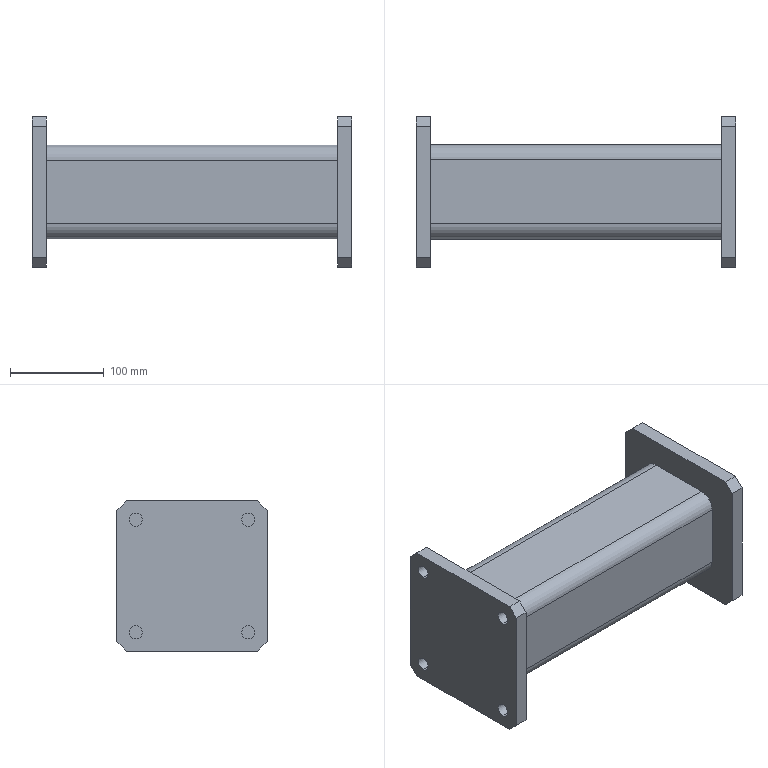Part | SolidWorks | features 3DProfileFeature 1, Extrusion 1, HoleWzd 1, ICE 1, MirrorPattern 1 | 1 solid | 46 faces | box 340 x 160 x 160 mm | volume 1614311 mm3 | plane 30 | cylinder 16 | commonest cylinder face diameters 14 x8 16 x4 32 x4
STEP:
#1=CARTESIAN_POINT('',(0.,140.,-133.));
#2=VERTEX_POINT('',#1);
#3=CARTESIAN_POINT('',(0.,140.,-147.));
#4=VERTEX_POINT('',#3);
#5=CARTESIAN_POINT('',(0.,140.,-140.));
#6=DIRECTION('',(1.,0.,0.));
#7=DIRECTION('',(0.,0.,-1.));
#8=AXIS2_PLACEMENT_3D('',#5,#6,#7);
#9=CIRCLE('',#8,7.);
#10=EDGE_CURVE('',#2,#4,#9,.T.);
#11=ORIENTED_EDGE('',*,*,#10,.F.);
#12=CARTESIAN_POINT('',(15.,140.,-133.));
#13=VERTEX_POINT('',#12);
#14=CARTESIAN_POINT('',(15.,140.,-133.));
#15=DIRECTION('',(1.,0.,0.));
#16=VECTOR('',#15,1000.);
#17=LINE('',#14,#16);
#18=EDGE_CURVE('',#2,#13,#17,.T.);
#19=ORIENTED_EDGE('',*,*,#18,.T.);
#20=CARTESIAN_POINT('',(15.,140.,-147.));
#21=VERTEX_POINT('',#20);
#22=CARTESIAN_POINT('',(15.,140.,-140.));
#23=DIRECTION('',(1.,0.,0.));
#24=DIRECTION('',(0.,0.,-1.));
#25=AXIS2_PLACEMENT_3D('',#22,#23,#24);
#26=CIRCLE('',#25,7.);
#27=EDGE_CURVE('',#13,#21,#26,.T.);
#28=ORIENTED_EDGE('',*,*,#27,.T.);
#29=CARTESIAN_POINT('',(15.,140.,-147.));
#30=DIRECTION('',(1.,0.,0.));
#31=VECTOR('',#30,1000.);
#32=LINE('',#29,#31);
#33=EDGE_CURVE('',#4,#21,#32,.T.);
#34=ORIENTED_EDGE('',*,*,#33,.F.);
#35=EDGE_LOOP('',(#11,#19,#28,#34));
#36=FACE_OUTER_BOUND('',#35,.T.);
#37=CARTESIAN_POINT('',(15.,140.,-140.));
#38=DIRECTION('',(1.,0.,0.));
#39=DIRECTION('',(0.,0.,-1.));
#40=AXIS2_PLACEMENT_3D('',#37,#38,#39);
#41=CYLINDRICAL_SURFACE('',#40,7.);
#42=ADVANCED_FACE('',(#36),#41,.F.);
#43=CARTESIAN_POINT('',(0.,20.,-133.));
#44=VERTEX_POINT('',#43);
#45=CARTESIAN_POINT('',(0.,20.,-147.));
#46=VERTEX_POINT('',#45);
#47=CARTESIAN_POINT('',(0.,20.,-140.));
#48=DIRECTION('',(1.,0.,0.));
#49=DIRECTION('',(0.,0.,-1.));
#50=AXIS2_PLACEMENT_3D('',#47,#48,#49);
#51=CIRCLE('',#50,7.);
#52=EDGE_CURVE('',#44,#46,#51,.T.);
#53=ORIENTED_EDGE('',*,*,#52,.F.);
#54=CARTESIAN_POINT('',(15.,20.,-133.));
#55=VERTEX_POINT('',#54);
#56=CARTESIAN_POINT('',(15.,20.,-133.));
#57=DIRECTION('',(1.,0.,0.));
#58=VECTOR('',#57,1000.);
#59=LINE('',#56,#58);
#60=EDGE_CURVE('',#44,#55,#59,.T.);
#61=ORIENTED_EDGE('',*,*,#60,.T.);
#62=CARTESIAN_POINT('',(15.,20.,-147.));
#63=VERTEX_POINT('',#62);
#64=CARTESIAN_POINT('',(15.,20.,-140.));
#65=DIRECTION('',(1.,0.,0.));
#66=DIRECTION('',(0.,0.,-1.));
#67=AXIS2_PLACEMENT_3D('',#64,#65,#66);
#68=CIRCLE('',#67,7.);
#69=EDGE_CURVE('',#55,#63,#68,.T.);
#70=ORIENTED_EDGE('',*,*,#69,.T.);
#71=CARTESIAN_POINT('',(15.,20.,-147.));
#72=DIRECTION('',(1.,0.,0.));
#73=VECTOR('',#72,1000.);
#74=LINE('',#71,#73);
#75=EDGE_CURVE('',#46,#63,#74,.T.);
#76=ORIENTED_EDGE('',*,*,#75,.F.);
#77=EDGE_LOOP('',(#53,#61,#70,#76));
#78=FACE_OUTER_BOUND('',#77,.T.);
#79=CARTESIAN_POINT('',(15.,20.,-140.));
#80=DIRECTION('',(1.,0.,0.));
#81=DIRECTION('',(0.,0.,-1.));
#82=AXIS2_PLACEMENT_3D('',#79,#80,#81);
#83=CYLINDRICAL_SURFACE('',#82,7.);
#84=ADVANCED_FACE('',(#78),#83,.F.);
#85=CARTESIAN_POINT('',(0.,140.,-13.));
#86=VERTEX_POINT('',#85);
#87=CARTESIAN_POINT('',(0.,140.,-27.));
#88=VERTEX_POINT('',#87);
#89=CARTESIAN_POINT('',(0.,140.,-20.));
#90=DIRECTION('',(1.,0.,0.));
#91=DIRECTION('',(0.,0.,-1.));
#92=AXIS2_PLACEMENT_3D('',#89,#90,#91);
#93=CIRCLE('',#92,7.);
#94=EDGE_CURVE('',#86,#88,#93,.T.);
#95=ORIENTED_EDGE('',*,*,#94,.F.);
#96=CARTESIAN_POINT('',(15.,140.,-13.));
#97=VERTEX_POINT('',#96);
#98=CARTESIAN_POINT('',(15.,140.,-13.));
#99=DIRECTION('',(1.,0.,0.));
#100=VECTOR('',#99,1000.);
#101=LINE('',#98,#100);
#102=EDGE_CURVE('',#86,#97,#101,.T.);
#103=ORIENTED_EDGE('',*,*,#102,.T.);
#104=CARTESIAN_POINT('',(15.,140.,-27.));
#105=VERTEX_POINT('',#104);
#106=CARTESIAN_POINT('',(15.,140.,-20.));
#107=DIRECTION('',(1.,0.,0.));
#108=DIRECTION('',(0.,0.,-1.));
#109=AXIS2_PLACEMENT_3D('',#106,#107,#108);
#110=CIRCLE('',#109,7.);
#111=EDGE_CURVE('',#97,#105,#110,.T.);
#112=ORIENTED_EDGE('',*,*,#111,.T.);
#113=CARTESIAN_POINT('',(15.,140.,-27.));
#114=DIRECTION('',(1.,0.,0.));
#115=VECTOR('',#114,1000.);
#116=LINE('',#113,#115);
#117=EDGE_CURVE('',#88,#105,#116,.T.);
#118=ORIENTED_EDGE('',*,*,#117,.F.);
#119=EDGE_LOOP('',(#95,#103,#112,#118));
#120=FACE_OUTER_BOUND('',#119,.T.);
#121=CARTESIAN_POINT('',(15.,140.,-20.));
#122=DIRECTION('',(1.,0.,0.));
#123=DIRECTION('',(0.,0.,-1.));
#124=AXIS2_PLACEMENT_3D('',#121,#122,#123);
#125=CYLINDRICAL_SURFACE('',#124,7.);
#126=ADVANCED_FACE('',(#120),#125,.F.);
#127=CARTESIAN_POINT('',(0.,20.,-13.));
#128=VERTEX_POINT('',#127);
#129=CARTESIAN_POINT('',(0.,20.,-27.));
#130=VERTEX_POINT('',#129);
#131=CARTESIAN_POINT('',(0.,20.,-20.));
#132=DIRECTION('',(1.,0.,0.));
#133=DIRECTION('',(0.,0.,-1.));
#134=AXIS2_PLACEMENT_3D('',#131,#132,#133);
#135=CIRCLE('',#134,7.);
#136=EDGE_CURVE('',#128,#130,#135,.T.);
#137=ORIENTED_EDGE('',*,*,#136,.F.);
#138=CARTESIAN_POINT('',(15.,20.,-13.));
#139=VERTEX_POINT('',#138);
#140=CARTESIAN_POINT('',(15.,20.,-13.));
#141=DIRECTION('',(1.,0.,0.));
#142=VECTOR('',#141,1000.);
#143=LINE('',#140,#142);
#144=EDGE_CURVE('',#128,#139,#143,.T.);
#145=ORIENTED_EDGE('',*,*,#144,.T.);
#146=CARTESIAN_POINT('',(15.,20.,-27.));
#147=VERTEX_POINT('',#146);
#148=CARTESIAN_POINT('',(15.,20.,-20.));
#149=DIRECTION('',(1.,0.,0.));
#150=DIRECTION('',(0.,0.,-1.));
#151=AXIS2_PLACEMENT_3D('',#148,#149,#150);
#152=CIRCLE('',#151,7.);
#153=EDGE_CURVE('',#139,#147,#152,.T.);
#154=ORIENTED_EDGE('',*,*,#153,.T.);
#155=CARTESIAN_POINT('',(15.,20.,-27.));
#156=DIRECTION('',(1.,0.,0.));
#157=VECTOR('',#156,1000.);
#158=LINE('',#155,#157);
#159=EDGE_CURVE('',#130,#147,#158,.T.);
#160=ORIENTED_EDGE('',*,*,#159,.F.);
#161=EDGE_LOOP('',(#137,#145,#154,#160));
#162=FACE_OUTER_BOUND('',#161,.T.);
#163=CARTESIAN_POINT('',(15.,20.,-20.));
#164=DIRECTION('',(1.,0.,0.));
#165=DIRECTION('',(0.,0.,-1.));
#166=AXIS2_PLACEMENT_3D('',#163,#164,#165);
#167=CYLINDRICAL_SURFACE('',#166,7.);
#168=ADVANCED_FACE('',(#162),#167,.F.);
#169=CARTESIAN_POINT('',(15.,140.,-140.));
#170=DIRECTION('',(1.,0.,0.));
#171=DIRECTION('',(0.,0.,-1.));
#172=AXIS2_PLACEMENT_3D('',#169,#170,#171);
#173=CIRCLE('',#172,7.);
#174=EDGE_CURVE('',#21,#13,#173,.T.);
#175=ORIENTED_EDGE('',*,*,#174,.F.);
#176=ORIENTED_EDGE('',*,*,#27,.F.);
#177=EDGE_LOOP('',(#175,#176));
#178=FACE_BOUND('',#177,.T.);
#179=CARTESIAN_POINT('',(15.,20.,-140.));
#180=DIRECTION('',(1.,0.,0.));
#181=DIRECTION('',(0.,0.,-1.));
#182=AXIS2_PLACEMENT_3D('',#179,#180,#181);
#183=CIRCLE('',#182,7.);
#184=EDGE_CURVE('',#63,#55,#183,.T.);
#185=ORIENTED_EDGE('',*,*,#184,.F.);
#186=ORIENTED_EDGE('',*,*,#69,.F.);
#187=EDGE_LOOP('',(#185,#186));
#188=FACE_BOUND('',#187,.T.);
#189=CARTESIAN_POINT('',(15.,140.,-20.));
#190=DIRECTION('',(1.,0.,0.));
#191=DIRECTION('',(0.,0.,-1.));
#192=AXIS2_PLACEMENT_3D('',#189,#190,#191);
#193=CIRCLE('',#192,7.);
#194=EDGE_CURVE('',#105,#97,#193,.T.);
#195=ORIENTED_EDGE('',*,*,#194,.F.);
#196=ORIENTED_EDGE('',*,*,#111,.F.);
#197=EDGE_LOOP('',(#195,#196));
#198=FACE_BOUND('',#197,.T.);
#199=CARTESIAN_POINT('',(15.,20.,-20.));
#200=DIRECTION('',(1.,0.,0.));
#201=DIRECTION('',(0.,0.,-1.));
#202=AXIS2_PLACEMENT_3D('',#199,#200,#201);
#203=CIRCLE('',#202,7.);
#204=EDGE_CURVE('',#147,#139,#203,.T.);
#205=ORIENTED_EDGE('',*,*,#204,.F.);
#206=ORIENTED_EDGE('',*,*,#153,.F.);
#207=EDGE_LOOP('',(#205,#206));
#208=FACE_BOUND('',#207,.T.);
#209=CARTESIAN_POINT('',(15.,160.,-150.));
#210=VERTEX_POINT('',#209);
#211=CARTESIAN_POINT('',(15.,160.,-10.));
#212=VERTEX_POINT('',#211);
#213=CARTESIAN_POINT('',(15.,160.,-10.));
#214=DIRECTION('',(0.,0.,1.));
#215=VECTOR('',#214,1000.);
#216=LINE('',#213,#215);
#217=EDGE_CURVE('',#210,#212,#216,.T.);
#218=ORIENTED_EDGE('',*,*,#217,.T.);
#219=CARTESIAN_POINT('',(15.,150.,0.));
#220=VERTEX_POINT('',#219);
#221=CARTESIAN_POINT('',(15.,150.,0.));
#222=DIRECTION('',(0.,-0.7071,0.7071));
#223=VECTOR('',#222,1000.);
#224=LINE('',#221,#223);
#225=EDGE_CURVE('',#212,#220,#224,.T.);
#226=ORIENTED_EDGE('',*,*,#225,.T.);
#227=CARTESIAN_POINT('',(15.,10.,0.));
#228=VERTEX_POINT('',#227);
#229=CARTESIAN_POINT('',(15.,10.,0.));
#230=DIRECTION('',(0.,-1.,0.));
#231=VECTOR('',#230,1000.);
#232=LINE('',#229,#231);
#233=EDGE_CURVE('',#220,#228,#232,.T.);
#234=ORIENTED_EDGE('',*,*,#233,.T.);
#235=CARTESIAN_POINT('',(15.,0.,-10.));
#236=VERTEX_POINT('',#235);
#237=CARTESIAN_POINT('',(15.,0.,-10.));
#238=DIRECTION('',(0.,-0.7071,-0.7071));
#239=VECTOR('',#238,1000.);
#240=LINE('',#237,#239);
#241=EDGE_CURVE('',#228,#236,#240,.T.);
#242=ORIENTED_EDGE('',*,*,#241,.T.);
#243=CARTESIAN_POINT('',(15.,0.,-150.));
#244=VERTEX_POINT('',#243);
#245=CARTESIAN_POINT('',(15.,0.,-10.));
#246=DIRECTION('',(0.,0.,-1.));
#247=VECTOR('',#246,1000.);
#248=LINE('',#245,#247);
#249=EDGE_CURVE('',#236,#244,#248,.T.);
#250=ORIENTED_EDGE('',*,*,#249,.T.);
#251=CARTESIAN_POINT('',(15.,10.,-160.));
#252=VERTEX_POINT('',#251);
#253=CARTESIAN_POINT('',(15.,0.,-150.));
#254=DIRECTION('',(0.,0.7071,-0.7071));
#255=VECTOR('',#254,1000.);
#256=LINE('',#253,#255);
#257=EDGE_CURVE('',#244,#252,#256,.T.);
#258=ORIENTED_EDGE('',*,*,#257,.T.);
#259=CARTESIAN_POINT('',(15.,150.,-160.));
#260=VERTEX_POINT('',#259);
#261=CARTESIAN_POINT('',(15.,10.,-160.));
#262=DIRECTION('',(0.,1.,0.));
#263=VECTOR('',#262,1000.);
#264=LINE('',#261,#263);
#265=EDGE_CURVE('',#252,#260,#264,.T.);
#266=ORIENTED_EDGE('',*,*,#265,.T.);
#267=CARTESIAN_POINT('',(15.,150.,-160.));
#268=DIRECTION('',(0.,0.7071,0.7071));
#269=VECTOR('',#268,1000.);
#270=LINE('',#267,#269);
#271=EDGE_CURVE('',#260,#210,#270,.T.);
#272=ORIENTED_EDGE('',*,*,#271,.T.);
#273=EDGE_LOOP('',(#218,#226,#234,#242,#250,#258,#266,#272));
#274=FACE_OUTER_BOUND('',#273,.T.);
#275=CARTESIAN_POINT('',(15.,130.,-114.));
#276=VERTEX_POINT('',#275);
#277=CARTESIAN_POINT('',(15.,130.,-46.));
#278=VERTEX_POINT('',#277);
#279=CARTESIAN_POINT('',(15.,130.,-46.));
#280=DIRECTION('',(0.,0.,1.));
#281=VECTOR('',#280,1000.);
#282=LINE('',#279,#281);
#283=EDGE_CURVE('',#276,#278,#282,.T.);
#284=ORIENTED_EDGE('',*,*,#283,.F.);
#285=CARTESIAN_POINT('',(15.,114.,-130.));
#286=VERTEX_POINT('',#285);
#287=CARTESIAN_POINT('',(15.,114.,-114.));
#288=DIRECTION('',(1.,0.,0.));
#289=DIRECTION('',(0.,0.,1.));
#290=AXIS2_PLACEMENT_3D('',#287,#288,#289);
#291=CIRCLE('',#290,16.);
#292=EDGE_CURVE('',#286,#276,#291,.T.);
#293=ORIENTED_EDGE('',*,*,#292,.F.);
#294=CARTESIAN_POINT('',(15.,46.,-130.));
#295=VERTEX_POINT('',#294);
#296=CARTESIAN_POINT('',(15.,114.,-130.));
#297=DIRECTION('',(0.,1.,0.));
#298=VECTOR('',#297,1000.);
#299=LINE('',#296,#298);
#300=EDGE_CURVE('',#295,#286,#299,.T.);
#301=ORIENTED_EDGE('',*,*,#300,.F.);
#302=CARTESIAN_POINT('',(15.,30.,-114.));
#303=VERTEX_POINT('',#302);
#304=CARTESIAN_POINT('',(15.,46.,-114.));
#305=DIRECTION('',(1.,0.,0.));
#306=DIRECTION('',(0.,0.,1.));
#307=AXIS2_PLACEMENT_3D('',#304,#305,#306);
#308=CIRCLE('',#307,16.);
#309=EDGE_CURVE('',#303,#295,#308,.T.);
#310=ORIENTED_EDGE('',*,*,#309,.F.);
#311=CARTESIAN_POINT('',(15.,30.,-46.));
#312=VERTEX_POINT('',#311);
#313=CARTESIAN_POINT('',(15.,30.,-46.));
#314=DIRECTION('',(0.,0.,-1.));
#315=VECTOR('',#314,1000.);
#316=LINE('',#313,#315);
#317=EDGE_CURVE('',#312,#303,#316,.T.);
#318=ORIENTED_EDGE('',*,*,#317,.F.);
#319=CARTESIAN_POINT('',(15.,46.,-30.));
#320=VERTEX_POINT('',#319);
#321=CARTESIAN_POINT('',(15.,46.,-46.));
#322=DIRECTION('',(1.,0.,0.));
#323=DIRECTION('',(0.,0.,1.));
#324=AXIS2_PLACEMENT_3D('',#321,#322,#323);
#325=CIRCLE('',#324,16.);
#326=EDGE_CURVE('',#320,#312,#325,.T.);
#327=ORIENTED_EDGE('',*,*,#326,.F.);
#328=CARTESIAN_POINT('',(15.,114.,-30.));
#329=VERTEX_POINT('',#328);
#330=CARTESIAN_POINT('',(15.,114.,-30.));
#331=DIRECTION('',(0.,-1.,0.));
#332=VECTOR('',#331,1000.);
#333=LINE('',#330,#332);
#334=EDGE_CURVE('',#329,#320,#333,.T.);
#335=ORIENTED_EDGE('',*,*,#334,.F.);
#336=CARTESIAN_POINT('',(15.,114.,-46.));
#337=DIRECTION('',(1.,0.,0.));
#338=DIRECTION('',(0.,0.,1.));
#339=AXIS2_PLACEMENT_3D('',#336,#337,#338);
#340=CIRCLE('',#339,16.);
#341=EDGE_CURVE('',#278,#329,#340,.T.);
#342=ORIENTED_EDGE('',*,*,#341,.F.);
#343=EDGE_LOOP('',(#284,#293,#301,#310,#318,#327,#335,#342));
#344=FACE_BOUND('',#343,.T.);
#345=CARTESIAN_POINT('',(15.,160.,-160.));
#346=DIRECTION('',(1.,0.,0.));
#347=DIRECTION('',(0.,0.,-1.));
#348=AXIS2_PLACEMENT_3D('',#345,#346,#347);
#349=PLANE('',#348);
#350=ADVANCED_FACE('',(#178,#188,#198,#208,#274,#344),#349,.T.);
#351=CARTESIAN_POINT('',(0.,160.,-150.));
#352=VERTEX_POINT('',#351);
#353=CARTESIAN_POINT('',(0.,160.,-10.));
#354=VERTEX_POINT('',#353);
#355=CARTESIAN_POINT('',(0.,160.,-10.));
#356=DIRECTION('',(0.,0.,1.));
#357=VECTOR('',#356,1000.);
#358=LINE('',#355,#357);
#359=EDGE_CURVE('',#352,#354,#358,.T.);
#360=ORIENTED_EDGE('',*,*,#359,.T.);
#361=CARTESIAN_POINT('',(15.,160.,-10.));
#362=DIRECTION('',(-1.,0.,0.));
#363=VECTOR('',#362,1000.);
#364=LINE('',#361,#363);
#365=EDGE_CURVE('',#212,#354,#364,.T.);
#366=ORIENTED_EDGE('',*,*,#365,.F.);
#367=ORIENTED_EDGE('',*,*,#217,.F.);
#368=CARTESIAN_POINT('',(15.,160.,-150.));
#369=DIRECTION('',(-1.,0.,0.));
#370=VECTOR('',#369,1000.);
#371=LINE('',#368,#370);
#372=EDGE_CURVE('',#210,#352,#371,.T.);
#373=ORIENTED_EDGE('',*,*,#372,.T.);
#374=EDGE_LOOP('',(#360,#366,#367,#373));
#375=FACE_OUTER_BOUND('',#374,.T.);
#376=CARTESIAN_POINT('',(15.,160.,-10.));
#377=DIRECTION('',(0.,-1.,0.));
#378=DIRECTION('',(0.,0.,-1.));
#379=AXIS2_PLACEMENT_3D('',#376,#377,#378);
#380=PLANE('',#379);
#381=ADVANCED_FACE('',(#375),#380,.F.);
#382=CARTESIAN_POINT('',(0.,150.,0.));
#383=VERTEX_POINT('',#382);
#384=CARTESIAN_POINT('',(0.,150.,0.));
#385=DIRECTION('',(0.,-0.7071,0.7071));
#386=VECTOR('',#385,1000.);
#387=LINE('',#384,#386);
#388=EDGE_CURVE('',#354,#383,#387,.T.);
#389=ORIENTED_EDGE('',*,*,#388,.T.);
#390=CARTESIAN_POINT('',(15.,150.,0.));
#391=DIRECTION('',(-1.,0.,0.));
#392=VECTOR('',#391,1000.);
#393=LINE('',#390,#392);
#394=EDGE_CURVE('',#220,#383,#393,.T.);
#395=ORIENTED_EDGE('',*,*,#394,.F.);
#396=ORIENTED_EDGE('',*,*,#225,.F.);
#397=ORIENTED_EDGE('',*,*,#365,.T.);
#398=EDGE_LOOP('',(#389,#395,#396,#397));
#399=FACE_OUTER_BOUND('',#398,.T.);
#400=CARTESIAN_POINT('',(15.,150.,0.));
#401=DIRECTION('',(0.,-0.7071,-0.7071));
#402=DIRECTION('',(0.,0.7071,-0.7071));
#403=AXIS2_PLACEMENT_3D('',#400,#401,#402);
#404=PLANE('',#403);
#405=ADVANCED_FACE('',(#399),#404,.F.);
#406=CARTESIAN_POINT('',(0.,10.,0.));
#407=VERTEX_POINT('',#406);
#408=CARTESIAN_POINT('',(0.,10.,0.));
#409=DIRECTION('',(0.,-1.,0.));
#410=VECTOR('',#409,1000.);
#411=LINE('',#408,#410);
#412=EDGE_CURVE('',#383,#407,#411,.T.);
#413=ORIENTED_EDGE('',*,*,#412,.T.);
#414=CARTESIAN_POINT('',(15.,10.,0.));
#415=DIRECTION('',(-1.,0.,0.));
#416=VECTOR('',#415,1000.);
#417=LINE('',#414,#416);
#418=EDGE_CURVE('',#228,#407,#417,.T.);
#419=ORIENTED_EDGE('',*,*,#418,.F.);
#420=ORIENTED_EDGE('',*,*,#233,.F.);
#421=ORIENTED_EDGE('',*,*,#394,.T.);
#422=EDGE_LOOP('',(#413,#419,#420,#421));
#423=FACE_OUTER_BOUND('',#422,.T.);
#424=CARTESIAN_POINT('',(15.,10.,0.));
#425=DIRECTION('',(0.,0.,-1.));
#426=DIRECTION('',(-1.,0.,0.));
#427=AXIS2_PLACEMENT_3D('',#424,#425,#426);
#428=PLANE('',#427);
#429=ADVANCED_FACE('',(#423),#428,.F.);
#430=CARTESIAN_POINT('',(0.,0.,-10.));
#431=VERTEX_POINT('',#430);
#432=CARTESIAN_POINT('',(0.,0.,-10.));
#433=DIRECTION('',(0.,-0.7071,-0.7071));
#434=VECTOR('',#433,1000.);
#435=LINE('',#432,#434);
#436=EDGE_CURVE('',#407,#431,#435,.T.);
#437=ORIENTED_EDGE('',*,*,#436,.T.);
#438=CARTESIAN_POINT('',(15.,0.,-10.));
#439=DIRECTION('',(-1.,0.,0.));
#440=VECTOR('',#439,1000.);
#441=LINE('',#438,#440);
#442=EDGE_CURVE('',#236,#431,#441,.T.);
#443=ORIENTED_EDGE('',*,*,#442,.F.);
#444=ORIENTED_EDGE('',*,*,#241,.F.);
#445=ORIENTED_EDGE('',*,*,#418,.T.);
#446=EDGE_LOOP('',(#437,#443,#444,#445));
#447=FACE_OUTER_BOUND('',#446,.T.);
#448=CARTESIAN_POINT('',(15.,0.,-10.));
#449=DIRECTION('',(0.,0.7071,-0.7071));
#450=DIRECTION('',(0.,0.7071,0.7071));
#451=AXIS2_PLACEMENT_3D('',#448,#449,#450);
#452=PLANE('',#451);
#453=ADVANCED_FACE('',(#447),#452,.F.);
#454=CARTESIAN_POINT('',(0.,0.,-150.));
#455=VERTEX_POINT('',#454);
#456=CARTESIAN_POINT('',(0.,0.,-10.));
#457=DIRECTION('',(0.,0.,-1.));
#458=VECTOR('',#457,1000.);
#459=LINE('',#456,#458);
#460=EDGE_CURVE('',#431,#455,#459,.T.);
#461=ORIENTED_EDGE('',*,*,#460,.T.);
#462=CARTESIAN_POINT('',(15.,0.,-150.));
#463=DIRECTION('',(-1.,0.,0.));
#464=VECTOR('',#463,1000.);
#465=LINE('',#462,#464);
#466=EDGE_CURVE('',#244,#455,#465,.T.);
#467=ORIENTED_EDGE('',*,*,#466,.F.);
#468=ORIENTED_EDGE('',*,*,#249,.F.);
#469=ORIENTED_EDGE('',*,*,#442,.T.);
#470=EDGE_LOOP('',(#461,#467,#468,#469));
#471=FACE_OUTER_BOUND('',#470,.T.);
#472=CARTESIAN_POINT('',(15.,0.,-10.));
#473=DIRECTION('',(0.,1.,0.));
#474=DIRECTION('',(0.,0.,1.));
#475=AXIS2_PLACEMENT_3D('',#472,#473,#474);
#476=PLANE('',#475);
#477=ADVANCED_FACE('',(#471),#476,.F.);
#478=CARTESIAN_POINT('',(0.,10.,-160.));
#479=VERTEX_POINT('',#478);
#480=CARTESIAN_POINT('',(0.,0.,-150.));
#481=DIRECTION('',(0.,0.7071,-0.7071));
#482=VECTOR('',#481,1000.);
#483=LINE('',#480,#482);
#484=EDGE_CURVE('',#455,#479,#483,.T.);
#485=ORIENTED_EDGE('',*,*,#484,.T.);
#486=CARTESIAN_POINT('',(15.,10.,-160.));
#487=DIRECTION('',(-1.,0.,0.));
#488=VECTOR('',#487,1000.);
#489=LINE('',#486,#488);
#490=EDGE_CURVE('',#252,#479,#489,.T.);
#491=ORIENTED_EDGE('',*,*,#490,.F.);
#492=ORIENTED_EDGE('',*,*,#257,.F.);
#493=ORIENTED_EDGE('',*,*,#466,.T.);
#494=EDGE_LOOP('',(#485,#491,#492,#493));
#495=FACE_OUTER_BOUND('',#494,.T.);
#496=CARTESIAN_POINT('',(15.,0.,-150.));
#497=DIRECTION('',(0.,0.7071,0.7071));
#498=DIRECTION('',(0.,-0.7071,0.7071));
#499=AXIS2_PLACEMENT_3D('',#496,#497,#498);
#500=PLANE('',#499);
#501=ADVANCED_FACE('',(#495),#500,.F.);
#502=CARTESIAN_POINT('',(0.,150.,-160.));
#503=VERTEX_POINT('',#502);
#504=CARTESIAN_POINT('',(0.,10.,-160.));
#505=DIRECTION('',(0.,1.,0.));
#506=VECTOR('',#505,1000.);
#507=LINE('',#504,#506);
#508=EDGE_CURVE('',#479,#503,#507,.T.);
#509=ORIENTED_EDGE('',*,*,#508,.T.);
#510=CARTESIAN_POINT('',(15.,150.,-160.));
#511=DIRECTION('',(-1.,0.,0.));
#512=VECTOR('',#511,1000.);
#513=LINE('',#510,#512);
#514=EDGE_CURVE('',#260,#503,#513,.T.);
#515=ORIENTED_EDGE('',*,*,#514,.F.);
#516=ORIENTED_EDGE('',*,*,#265,.F.);
#517=ORIENTED_EDGE('',*,*,#490,.T.);
#518=EDGE_LOOP('',(#509,#515,#516,#517));
#519=FACE_OUTER_BOUND('',#518,.T.);
#520=CARTESIAN_POINT('',(15.,10.,-160.));
#521=DIRECTION('',(0.,0.,1.));
#522=DIRECTION('',(1.,0.,0.));
#523=AXIS2_PLACEMENT_3D('',#520,#521,#522);
#524=PLANE('',#523);
#525=ADVANCED_FACE('',(#519),#524,.F.);
#526=CARTESIAN_POINT('',(0.,150.,-160.));
#527=DIRECTION('',(0.,0.7071,0.7071));
#528=VECTOR('',#527,1000.);
#529=LINE('',#526,#528);
#530=EDGE_CURVE('',#503,#352,#529,.T.);
#531=ORIENTED_EDGE('',*,*,#530,.T.);
#532=ORIENTED_EDGE('',*,*,#372,.F.);
#533=ORIENTED_EDGE('',*,*,#271,.F.);
#534=ORIENTED_EDGE('',*,*,#514,.T.);
#535=EDGE_LOOP('',(#531,#532,#533,#534));
#536=FACE_OUTER_BOUND('',#535,.T.);
#537=CARTESIAN_POINT('',(15.,150.,-160.));
#538=DIRECTION('',(0.,-0.7071,0.7071));
#539=DIRECTION('',(0.,-0.7071,-0.7071));
#540=AXIS2_PLACEMENT_3D('',#537,#538,#539);
#541=PLANE('',#540);
#542=ADVANCED_FACE('',(#536),#541,.F.);
#543=CARTESIAN_POINT('',(0.,140.,-140.));
#544=DIRECTION('',(1.,0.,0.));
#545=DIRECTION('',(0.,0.,-1.));
#546=AXIS2_PLACEMENT_3D('',#543,#544,#545);
#547=CIRCLE('',#546,7.);
#548=EDGE_CURVE('',#4,#2,#547,.T.);
#549=ORIENTED_EDGE('',*,*,#548,.T.);
#550=ORIENTED_EDGE('',*,*,#10,.T.);
#551=EDGE_LOOP('',(#549,#550));
#552=FACE_BOUND('',#551,.T.);
#553=CARTESIAN_POINT('',(0.,20.,-140.));
#554=DIRECTION('',(1.,0.,0.));
#555=DIRECTION('',(0.,0.,-1.));
#556=AXIS2_PLACEMENT_3D('',#553,#554,#555);
#557=CIRCLE('',#556,7.);
#558=EDGE_CURVE('',#46,#44,#557,.T.);
#559=ORIENTED_EDGE('',*,*,#558,.T.);
#560=ORIENTED_EDGE('',*,*,#52,.T.);
#561=EDGE_LOOP('',(#559,#560));
#562=FACE_BOUND('',#561,.T.);
#563=CARTESIAN_POINT('',(0.,140.,-20.));
#564=DIRECTION('',(1.,0.,0.));
#565=DIRECTION('',(0.,0.,-1.));
#566=AXIS2_PLACEMENT_3D('',#563,#564,#565);
#567=CIRCLE('',#566,7.);
#568=EDGE_CURVE('',#88,#86,#567,.T.);
#569=ORIENTED_EDGE('',*,*,#568,.T.);
#570=ORIENTED_EDGE('',*,*,#94,.T.);
#571=EDGE_LOOP('',(#569,#570));
#572=FACE_BOUND('',#571,.T.);
#573=CARTESIAN_POINT('',(0.,20.,-20.));
#574=DIRECTION('',(1.,0.,0.));
#575=DIRECTION('',(0.,0.,-1.));
#576=AXIS2_PLACEMENT_3D('',#573,#574,#575);
#577=CIRCLE('',#576,7.);
#578=EDGE_CURVE('',#130,#128,#577,.T.);
#579=ORIENTED_EDGE('',*,*,#578,.T.);
#580=ORIENTED_EDGE('',*,*,#136,.T.);
#581=EDGE_LOOP('',(#579,#580));
#582=FACE_BOUND('',#581,.T.);
#583=ORIENTED_EDGE('',*,*,#359,.F.);
#584=ORIENTED_EDGE('',*,*,#530,.F.);
#585=ORIENTED_EDGE('',*,*,#508,.F.);
#586=ORIENTED_EDGE('',*,*,#484,.F.);
#587=ORIENTED_EDGE('',*,*,#460,.F.);
#588=ORIENTED_EDGE('',*,*,#436,.F.);
#589=ORIENTED_EDGE('',*,*,#412,.F.);
#590=ORIENTED_EDGE('',*,*,#388,.F.);
#591=EDGE_LOOP('',(#583,#584,#585,#586,#587,#588,#589,#590));
#592=FACE_OUTER_BOUND('',#591,.T.);
#593=CARTESIAN_POINT('',(0.,160.,-160.));
#594=DIRECTION('',(1.,0.,0.));
#595=DIRECTION('',(0.,0.,-1.));
#596=AXIS2_PLACEMENT_3D('',#593,#594,#595);
#597=PLANE('',#596);
#598=ADVANCED_FACE('',(#552,#562,#572,#582,#592),#597,.F.);
#599=ORIENTED_EDGE('',*,*,#292,.T.);
#600=CARTESIAN_POINT('',(325.,130.,-114.));
#601=VERTEX_POINT('',#600);
#602=CARTESIAN_POINT('',(325.,130.,-114.));
#603=DIRECTION('',(-1.,0.,0.));
#604=VECTOR('',#603,1000.);
#605=LINE('',#602,#604);
#606=EDGE_CURVE('',#601,#276,#605,.T.);
#607=ORIENTED_EDGE('',*,*,#606,.F.);
#608=CARTESIAN_POINT('',(325.,114.,-130.));
#609=VERTEX_POINT('',#608);
#610=CARTESIAN_POINT('',(325.,114.,-114.));
#611=DIRECTION('',(1.,0.,0.));
#612=DIRECTION('',(0.,0.,1.));
#613=AXIS2_PLACEMENT_3D('',#610,#611,#612);
#614=CIRCLE('',#613,16.);
#615=EDGE_CURVE('',#609,#601,#614,.T.);
#616=ORIENTED_EDGE('',*,*,#615,.F.);
#617=CARTESIAN_POINT('',(325.,114.,-130.));
#618=DIRECTION('',(-1.,0.,0.));
#619=VECTOR('',#618,1000.);
#620=LINE('',#617,#619);
#621=EDGE_CURVE('',#609,#286,#620,.T.);
#622=ORIENTED_EDGE('',*,*,#621,.T.);
#623=EDGE_LOOP('',(#599,#607,#616,#622));
#624=FACE_OUTER_BOUND('',#623,.T.);
#625=CARTESIAN_POINT('',(325.,114.,-114.));
#626=DIRECTION('',(-1.,0.,0.));
#627=DIRECTION('',(0.,0.,1.));
#628=AXIS2_PLACEMENT_3D('',#625,#626,#627);
#629=CYLINDRICAL_SURFACE('',#628,16.);
#630=ADVANCED_FACE('',(#624),#629,.T.);
#631=ORIENTED_EDGE('',*,*,#283,.T.);
#632=CARTESIAN_POINT('',(325.,130.,-46.));
#633=VERTEX_POINT('',#632);
#634=CARTESIAN_POINT('',(325.,130.,-46.));
#635=DIRECTION('',(-1.,0.,0.));
#636=VECTOR('',#635,1000.);
#637=LINE('',#634,#636);
#638=EDGE_CURVE('',#633,#278,#637,.T.);
#639=ORIENTED_EDGE('',*,*,#638,.F.);
#640=CARTESIAN_POINT('',(325.,130.,-46.));
#641=DIRECTION('',(0.,0.,1.));
#642=VECTOR('',#641,1000.);
#643=LINE('',#640,#642);
#644=EDGE_CURVE('',#601,#633,#643,.T.);
#645=ORIENTED_EDGE('',*,*,#644,.F.);
#646=ORIENTED_EDGE('',*,*,#606,.T.);
#647=EDGE_LOOP('',(#631,#639,#645,#646));
#648=FACE_OUTER_BOUND('',#647,.T.);
#649=CARTESIAN_POINT('',(325.,130.,-46.));
#650=DIRECTION('',(0.,-1.,0.));
#651=DIRECTION('',(0.,0.,-1.));
#652=AXIS2_PLACEMENT_3D('',#649,#650,#651);
#653=PLANE('',#652);
#654=ADVANCED_FACE('',(#648),#653,.F.);
#655=ORIENTED_EDGE('',*,*,#341,.T.);
#656=CARTESIAN_POINT('',(325.,114.,-30.));
#657=VERTEX_POINT('',#656);
#658=CARTESIAN_POINT('',(325.,114.,-30.));
#659=DIRECTION('',(-1.,0.,0.));
#660=VECTOR('',#659,1000.);
#661=LINE('',#658,#660);
#662=EDGE_CURVE('',#657,#329,#661,.T.);
#663=ORIENTED_EDGE('',*,*,#662,.F.);
#664=CARTESIAN_POINT('',(325.,114.,-46.));
#665=DIRECTION('',(1.,0.,0.));
#666=DIRECTION('',(0.,0.,1.));
#667=AXIS2_PLACEMENT_3D('',#664,#665,#666);
#668=CIRCLE('',#667,16.);
#669=EDGE_CURVE('',#633,#657,#668,.T.);
#670=ORIENTED_EDGE('',*,*,#669,.F.);
#671=ORIENTED_EDGE('',*,*,#638,.T.);
#672=EDGE_LOOP('',(#655,#663,#670,#671));
#673=FACE_OUTER_BOUND('',#672,.T.);
#674=CARTESIAN_POINT('',(325.,114.,-46.));
#675=DIRECTION('',(-1.,0.,0.));
#676=DIRECTION('',(0.,0.,1.));
#677=AXIS2_PLACEMENT_3D('',#674,#675,#676);
#678=CYLINDRICAL_SURFACE('',#677,16.);
#679=ADVANCED_FACE('',(#673),#678,.T.);
#680=ORIENTED_EDGE('',*,*,#334,.T.);
#681=CARTESIAN_POINT('',(325.,46.,-30.));
#682=VERTEX_POINT('',#681);
#683=CARTESIAN_POINT('',(325.,46.,-30.));
#684=DIRECTION('',(-1.,0.,0.));
#685=VECTOR('',#684,1000.);
#686=LINE('',#683,#685);
#687=EDGE_CURVE('',#682,#320,#686,.T.);
#688=ORIENTED_EDGE('',*,*,#687,.F.);
#689=CARTESIAN_POINT('',(325.,114.,-30.));
#690=DIRECTION('',(0.,-1.,0.));
#691=VECTOR('',#690,1000.);
#692=LINE('',#689,#691);
#693=EDGE_CURVE('',#657,#682,#692,.T.);
#694=ORIENTED_EDGE('',*,*,#693,.F.);
#695=ORIENTED_EDGE('',*,*,#662,.T.);
#696=EDGE_LOOP('',(#680,#688,#694,#695));
#697=FACE_OUTER_BOUND('',#696,.T.);
#698=CARTESIAN_POINT('',(325.,114.,-30.));
#699=DIRECTION('',(0.,0.,-1.));
#700=DIRECTION('',(0.,1.,0.));
#701=AXIS2_PLACEMENT_3D('',#698,#699,#700);
#702=PLANE('',#701);
#703=ADVANCED_FACE('',(#697),#702,.F.);
#704=ORIENTED_EDGE('',*,*,#326,.T.);
#705=CARTESIAN_POINT('',(325.,30.,-46.));
#706=VERTEX_POINT('',#705);
#707=CARTESIAN_POINT('',(325.,30.,-46.));
#708=DIRECTION('',(-1.,0.,0.));
#709=VECTOR('',#708,1000.);
#710=LINE('',#707,#709);
#711=EDGE_CURVE('',#706,#312,#710,.T.);
#712=ORIENTED_EDGE('',*,*,#711,.F.);
#713=CARTESIAN_POINT('',(325.,46.,-46.));
#714=DIRECTION('',(1.,0.,0.));
#715=DIRECTION('',(0.,0.,1.));
#716=AXIS2_PLACEMENT_3D('',#713,#714,#715);
#717=CIRCLE('',#716,16.);
#718=EDGE_CURVE('',#682,#706,#717,.T.);
#719=ORIENTED_EDGE('',*,*,#718,.F.);
#720=ORIENTED_EDGE('',*,*,#687,.T.);
#721=EDGE_LOOP('',(#704,#712,#719,#720));
#722=FACE_OUTER_BOUND('',#721,.T.);
#723=CARTESIAN_POINT('',(325.,46.,-46.));
#724=DIRECTION('',(-1.,0.,0.));
#725=DIRECTION('',(0.,0.,1.));
#726=AXIS2_PLACEMENT_3D('',#723,#724,#725);
#727=CYLINDRICAL_SURFACE('',#726,16.);
#728=ADVANCED_FACE('',(#722),#727,.T.);
#729=ORIENTED_EDGE('',*,*,#317,.T.);
#730=CARTESIAN_POINT('',(325.,30.,-114.));
#731=VERTEX_POINT('',#730);
#732=CARTESIAN_POINT('',(325.,30.,-114.));
#733=DIRECTION('',(-1.,0.,0.));
#734=VECTOR('',#733,1000.);
#735=LINE('',#732,#734);
#736=EDGE_CURVE('',#731,#303,#735,.T.);
#737=ORIENTED_EDGE('',*,*,#736,.F.);
#738=CARTESIAN_POINT('',(325.,30.,-46.));
#739=DIRECTION('',(0.,0.,-1.));
#740=VECTOR('',#739,1000.);
#741=LINE('',#738,#740);
#742=EDGE_CURVE('',#706,#731,#741,.T.);
#743=ORIENTED_EDGE('',*,*,#742,.F.);
#744=ORIENTED_EDGE('',*,*,#711,.T.);
#745=EDGE_LOOP('',(#729,#737,#743,#744));
#746=FACE_OUTER_BOUND('',#745,.T.);
#747=CARTESIAN_POINT('',(325.,30.,-46.));
#748=DIRECTION('',(0.,1.,0.));
#749=DIRECTION('',(0.,0.,1.));
#750=AXIS2_PLACEMENT_3D('',#747,#748,#749);
#751=PLANE('',#750);
#752=ADVANCED_FACE('',(#746),#751,.F.);
#753=ORIENTED_EDGE('',*,*,#309,.T.);
#754=CARTESIAN_POINT('',(325.,46.,-130.));
#755=VERTEX_POINT('',#754);
#756=CARTESIAN_POINT('',(325.,46.,-130.));
#757=DIRECTION('',(-1.,0.,0.));
#758=VECTOR('',#757,1000.);
#759=LINE('',#756,#758);
#760=EDGE_CURVE('',#755,#295,#759,.T.);
#761=ORIENTED_EDGE('',*,*,#760,.F.);
#762=CARTESIAN_POINT('',(325.,46.,-114.));
#763=DIRECTION('',(1.,0.,0.));
#764=DIRECTION('',(0.,0.,1.));
#765=AXIS2_PLACEMENT_3D('',#762,#763,#764);
#766=CIRCLE('',#765,16.);
#767=EDGE_CURVE('',#731,#755,#766,.T.);
#768=ORIENTED_EDGE('',*,*,#767,.F.);
#769=ORIENTED_EDGE('',*,*,#736,.T.);
#770=EDGE_LOOP('',(#753,#761,#768,#769));
#771=FACE_OUTER_BOUND('',#770,.T.);
#772=CARTESIAN_POINT('',(325.,46.,-114.));
#773=DIRECTION('',(-1.,0.,0.));
#774=DIRECTION('',(0.,0.,1.));
#775=AXIS2_PLACEMENT_3D('',#772,#773,#774);
#776=CYLINDRICAL_SURFACE('',#775,16.);
#777=ADVANCED_FACE('',(#771),#776,.T.);
#778=ORIENTED_EDGE('',*,*,#300,.T.);
#779=ORIENTED_EDGE('',*,*,#621,.F.);
#780=CARTESIAN_POINT('',(325.,114.,-130.));
#781=DIRECTION('',(0.,1.,0.));
#782=VECTOR('',#781,1000.);
#783=LINE('',#780,#782);
#784=EDGE_CURVE('',#755,#609,#783,.T.);
#785=ORIENTED_EDGE('',*,*,#784,.F.);
#786=ORIENTED_EDGE('',*,*,#760,.T.);
#787=EDGE_LOOP('',(#778,#779,#785,#786));
#788=FACE_OUTER_BOUND('',#787,.T.);
#789=CARTESIAN_POINT('',(325.,114.,-130.));
#790=DIRECTION('',(0.,0.,1.));
#791=DIRECTION('',(0.,-1.,0.));
#792=AXIS2_PLACEMENT_3D('',#789,#790,#791);
#793=PLANE('',#792);
#794=ADVANCED_FACE('',(#788),#793,.F.);
#795=CARTESIAN_POINT('',(325.,160.,-150.));
#796=VERTEX_POINT('',#795);
#797=CARTESIAN_POINT('',(325.,160.,-10.));
#798=VERTEX_POINT('',#797);
#799=CARTESIAN_POINT('',(325.,160.,-10.));
#800=DIRECTION('',(0.,0.,1.));
#801=VECTOR('',#800,1000.);
#802=LINE('',#799,#801);
#803=EDGE_CURVE('',#796,#798,#802,.T.);
#804=ORIENTED_EDGE('',*,*,#803,.F.);
#805=CARTESIAN_POINT('',(325.,150.,-160.));
#806=VERTEX_POINT('',#805);
#807=CARTESIAN_POINT('',(325.,150.,-160.));
#808=DIRECTION('',(0.,0.7071,0.7071));
#809=VECTOR('',#808,1000.);
#810=LINE('',#807,#809);
#811=EDGE_CURVE('',#806,#796,#810,.T.);
#812=ORIENTED_EDGE('',*,*,#811,.F.);
#813=CARTESIAN_POINT('',(325.,10.,-160.));
#814=VERTEX_POINT('',#813);
#815=CARTESIAN_POINT('',(325.,10.,-160.));
#816=DIRECTION('',(0.,1.,0.));
#817=VECTOR('',#816,1000.);
#818=LINE('',#815,#817);
#819=EDGE_CURVE('',#814,#806,#818,.T.);
#820=ORIENTED_EDGE('',*,*,#819,.F.);
#821=CARTESIAN_POINT('',(325.,0.,-150.));
#822=VERTEX_POINT('',#821);
#823=CARTESIAN_POINT('',(325.,0.,-150.));
#824=DIRECTION('',(0.,0.7071,-0.7071));
#825=VECTOR('',#824,1000.);
#826=LINE('',#823,#825);
#827=EDGE_CURVE('',#822,#814,#826,.T.);
#828=ORIENTED_EDGE('',*,*,#827,.F.);
#829=CARTESIAN_POINT('',(325.,0.,-10.));
#830=VERTEX_POINT('',#829);
#831=CARTESIAN_POINT('',(325.,0.,-10.));
#832=DIRECTION('',(0.,0.,-1.));
#833=VECTOR('',#832,1000.);
#834=LINE('',#831,#833);
#835=EDGE_CURVE('',#830,#822,#834,.T.);
#836=ORIENTED_EDGE('',*,*,#835,.F.);
#837=CARTESIAN_POINT('',(325.,10.,0.));
#838=VERTEX_POINT('',#837);
#839=CARTESIAN_POINT('',(325.,0.,-10.));
#840=DIRECTION('',(0.,-0.7071,-0.7071));
#841=VECTOR('',#840,1000.);
#842=LINE('',#839,#841);
#843=EDGE_CURVE('',#838,#830,#842,.T.);
#844=ORIENTED_EDGE('',*,*,#843,.F.);
#845=CARTESIAN_POINT('',(325.,150.,0.));
#846=VERTEX_POINT('',#845);
#847=CARTESIAN_POINT('',(325.,10.,0.));
#848=DIRECTION('',(0.,-1.,0.));
#849=VECTOR('',#848,1000.);
#850=LINE('',#847,#849);
#851=EDGE_CURVE('',#846,#838,#850,.T.);
#852=ORIENTED_EDGE('',*,*,#851,.F.);
#853=CARTESIAN_POINT('',(325.,150.,0.));
#854=DIRECTION('',(0.,-0.7071,0.7071));
#855=VECTOR('',#854,1000.);
#856=LINE('',#853,#855);
#857=EDGE_CURVE('',#798,#846,#856,.T.);
#858=ORIENTED_EDGE('',*,*,#857,.F.);
#859=EDGE_LOOP('',(#804,#812,#820,#828,#836,#844,#852,#858));
#860=FACE_OUTER_BOUND('',#859,.T.);
#861=ORIENTED_EDGE('',*,*,#615,.T.);
#862=ORIENTED_EDGE('',*,*,#644,.T.);
#863=ORIENTED_EDGE('',*,*,#669,.T.);
#864=ORIENTED_EDGE('',*,*,#693,.T.);
#865=ORIENTED_EDGE('',*,*,#718,.T.);
#866=ORIENTED_EDGE('',*,*,#742,.T.);
#867=ORIENTED_EDGE('',*,*,#767,.T.);
#868=ORIENTED_EDGE('',*,*,#784,.T.);
#869=EDGE_LOOP('',(#861,#862,#863,#864,#865,#866,#867,#868));
#870=FACE_BOUND('',#869,.T.);
#871=CARTESIAN_POINT('',(325.,160.,-160.));
#872=DIRECTION('',(-1.,0.,0.));
#873=DIRECTION('',(0.,0.,-1.));
#874=AXIS2_PLACEMENT_3D('',#871,#872,#873);
#875=PLANE('',#874);
#876=ADVANCED_FACE('',(#860,#870),#875,.T.);
#877=CARTESIAN_POINT('',(340.,160.,-150.));
#878=VERTEX_POINT('',#877);
#879=CARTESIAN_POINT('',(340.,160.,-10.));
#880=VERTEX_POINT('',#879);
#881=CARTESIAN_POINT('',(340.,160.,-10.));
#882=DIRECTION('',(0.,0.,1.));
#883=VECTOR('',#882,1000.);
#884=LINE('',#881,#883);
#885=EDGE_CURVE('',#878,#880,#884,.T.);
#886=ORIENTED_EDGE('',*,*,#885,.F.);
#887=CARTESIAN_POINT('',(325.,160.,-150.));
#888=DIRECTION('',(1.,0.,0.));
#889=VECTOR('',#888,1000.);
#890=LINE('',#887,#889);
#891=EDGE_CURVE('',#796,#878,#890,.T.);
#892=ORIENTED_EDGE('',*,*,#891,.F.);
#893=ORIENTED_EDGE('',*,*,#803,.T.);
#894=CARTESIAN_POINT('',(325.,160.,-10.));
#895=DIRECTION('',(1.,0.,0.));
#896=VECTOR('',#895,1000.);
#897=LINE('',#894,#896);
#898=EDGE_CURVE('',#798,#880,#897,.T.);
#899=ORIENTED_EDGE('',*,*,#898,.T.);
#900=EDGE_LOOP('',(#886,#892,#893,#899));
#901=FACE_OUTER_BOUND('',#900,.T.);
#902=CARTESIAN_POINT('',(325.,160.,-10.));
#903=DIRECTION('',(0.,1.,0.));
#904=DIRECTION('',(0.,0.,1.));
#905=AXIS2_PLACEMENT_3D('',#902,#903,#904);
#906=PLANE('',#905);
#907=ADVANCED_FACE('',(#901),#906,.T.);
#908=CARTESIAN_POINT('',(340.,150.,-160.));
#909=VERTEX_POINT('',#908);
#910=CARTESIAN_POINT('',(340.,150.,-160.));
#911=DIRECTION('',(0.,0.7071,0.7071));
#912=VECTOR('',#911,1000.);
#913=LINE('',#910,#912);
#914=EDGE_CURVE('',#909,#878,#913,.T.);
#915=ORIENTED_EDGE('',*,*,#914,.F.);
#916=CARTESIAN_POINT('',(325.,150.,-160.));
#917=DIRECTION('',(1.,0.,0.));
#918=VECTOR('',#917,1000.);
#919=LINE('',#916,#918);
#920=EDGE_CURVE('',#806,#909,#919,.T.);
#921=ORIENTED_EDGE('',*,*,#920,.F.);
#922=ORIENTED_EDGE('',*,*,#811,.T.);
#923=ORIENTED_EDGE('',*,*,#891,.T.);
#924=EDGE_LOOP('',(#915,#921,#922,#923));
#925=FACE_OUTER_BOUND('',#924,.T.);
#926=CARTESIAN_POINT('',(325.,150.,-160.));
#927=DIRECTION('',(0.,0.7071,-0.7071));
#928=DIRECTION('',(0.,0.7071,0.7071));
#929=AXIS2_PLACEMENT_3D('',#926,#927,#928);
#930=PLANE('',#929);
#931=ADVANCED_FACE('',(#925),#930,.T.);
#932=CARTESIAN_POINT('',(340.,10.,-160.));
#933=VERTEX_POINT('',#932);
#934=CARTESIAN_POINT('',(340.,10.,-160.));
#935=DIRECTION('',(0.,1.,0.));
#936=VECTOR('',#935,1000.);
#937=LINE('',#934,#936);
#938=EDGE_CURVE('',#933,#909,#937,.T.);
#939=ORIENTED_EDGE('',*,*,#938,.F.);
#940=CARTESIAN_POINT('',(325.,10.,-160.));
#941=DIRECTION('',(1.,0.,0.));
#942=VECTOR('',#941,1000.);
#943=LINE('',#940,#942);
#944=EDGE_CURVE('',#814,#933,#943,.T.);
#945=ORIENTED_EDGE('',*,*,#944,.F.);
#946=ORIENTED_EDGE('',*,*,#819,.T.);
#947=ORIENTED_EDGE('',*,*,#920,.T.);
#948=EDGE_LOOP('',(#939,#945,#946,#947));
#949=FACE_OUTER_BOUND('',#948,.T.);
#950=CARTESIAN_POINT('',(325.,10.,-160.));
#951=DIRECTION('',(0.,0.,-1.));
#952=DIRECTION('',(-1.,0.,0.));
#953=AXIS2_PLACEMENT_3D('',#950,#951,#952);
#954=PLANE('',#953);
#955=ADVANCED_FACE('',(#949),#954,.T.);
#956=CARTESIAN_POINT('',(340.,0.,-150.));
#957=VERTEX_POINT('',#956);
#958=CARTESIAN_POINT('',(340.,0.,-150.));
#959=DIRECTION('',(0.,0.7071,-0.7071));
#960=VECTOR('',#959,1000.);
#961=LINE('',#958,#960);
#962=EDGE_CURVE('',#957,#933,#961,.T.);
#963=ORIENTED_EDGE('',*,*,#962,.F.);
#964=CARTESIAN_POINT('',(325.,0.,-150.));
#965=DIRECTION('',(1.,0.,0.));
#966=VECTOR('',#965,1000.);
#967=LINE('',#964,#966);
#968=EDGE_CURVE('',#822,#957,#967,.T.);
#969=ORIENTED_EDGE('',*,*,#968,.F.);
#970=ORIENTED_EDGE('',*,*,#827,.T.);
#971=ORIENTED_EDGE('',*,*,#944,.T.);
#972=EDGE_LOOP('',(#963,#969,#970,#971));
#973=FACE_OUTER_BOUND('',#972,.T.);
#974=CARTESIAN_POINT('',(325.,0.,-150.));
#975=DIRECTION('',(0.,-0.7071,-0.7071));
#976=DIRECTION('',(0.,0.7071,-0.7071));
#977=AXIS2_PLACEMENT_3D('',#974,#975,#976);
#978=PLANE('',#977);
#979=ADVANCED_FACE('',(#973),#978,.T.);
#980=CARTESIAN_POINT('',(340.,0.,-10.));
#981=VERTEX_POINT('',#980);
#982=CARTESIAN_POINT('',(340.,0.,-10.));
#983=DIRECTION('',(0.,0.,-1.));
#984=VECTOR('',#983,1000.);
#985=LINE('',#982,#984);
#986=EDGE_CURVE('',#981,#957,#985,.T.);
#987=ORIENTED_EDGE('',*,*,#986,.F.);
#988=CARTESIAN_POINT('',(325.,0.,-10.));
#989=DIRECTION('',(1.,0.,0.));
#990=VECTOR('',#989,1000.);
#991=LINE('',#988,#990);
#992=EDGE_CURVE('',#830,#981,#991,.T.);
#993=ORIENTED_EDGE('',*,*,#992,.F.);
#994=ORIENTED_EDGE('',*,*,#835,.T.);
#995=ORIENTED_EDGE('',*,*,#968,.T.);
#996=EDGE_LOOP('',(#987,#993,#994,#995));
#997=FACE_OUTER_BOUND('',#996,.T.);
#998=CARTESIAN_POINT('',(325.,0.,-10.));
#999=DIRECTION('',(0.,-1.,0.));
#1000=DIRECTION('',(0.,0.,-1.));
#1001=AXIS2_PLACEMENT_3D('',#998,#999,#1000);
#1002=PLANE('',#1001);
#1003=ADVANCED_FACE('',(#997),#1002,.T.);
#1004=CARTESIAN_POINT('',(340.,10.,0.));
#1005=VERTEX_POINT('',#1004);
#1006=CARTESIAN_POINT('',(340.,0.,-10.));
#1007=DIRECTION('',(0.,-0.7071,-0.7071));
#1008=VECTOR('',#1007,1000.);
#1009=LINE('',#1006,#1008);
#1010=EDGE_CURVE('',#1005,#981,#1009,.T.);
#1011=ORIENTED_EDGE('',*,*,#1010,.F.);
#1012=CARTESIAN_POINT('',(325.,10.,0.));
#1013=DIRECTION('',(1.,0.,0.));
#1014=VECTOR('',#1013,1000.);
#1015=LINE('',#1012,#1014);
#1016=EDGE_CURVE('',#838,#1005,#1015,.T.);
#1017=ORIENTED_EDGE('',*,*,#1016,.F.);
#1018=ORIENTED_EDGE('',*,*,#843,.T.);
#1019=ORIENTED_EDGE('',*,*,#992,.T.);
#1020=EDGE_LOOP('',(#1011,#1017,#1018,#1019));
#1021=FACE_OUTER_BOUND('',#1020,.T.);
#1022=CARTESIAN_POINT('',(325.,0.,-10.));
#1023=DIRECTION('',(0.,-0.7071,0.7071));
#1024=DIRECTION('',(0.,-0.7071,-0.7071));
#1025=AXIS2_PLACEMENT_3D('',#1022,#1023,#1024);
#1026=PLANE('',#1025);
#1027=ADVANCED_FACE('',(#1021),#1026,.T.);
#1028=CARTESIAN_POINT('',(340.,150.,0.));
#1029=VERTEX_POINT('',#1028);
#1030=CARTESIAN_POINT('',(340.,10.,0.));
#1031=DIRECTION('',(0.,-1.,0.));
#1032=VECTOR('',#1031,1000.);
#1033=LINE('',#1030,#1032);
#1034=EDGE_CURVE('',#1029,#1005,#1033,.T.);
#1035=ORIENTED_EDGE('',*,*,#1034,.F.);
#1036=CARTESIAN_POINT('',(325.,150.,0.));
#1037=DIRECTION('',(1.,0.,0.));
#1038=VECTOR('',#1037,1000.);
#1039=LINE('',#1036,#1038);
#1040=EDGE_CURVE('',#846,#1029,#1039,.T.);
#1041=ORIENTED_EDGE('',*,*,#1040,.F.);
#1042=ORIENTED_EDGE('',*,*,#851,.T.);
#1043=ORIENTED_EDGE('',*,*,#1016,.T.);
#1044=EDGE_LOOP('',(#1035,#1041,#1042,#1043));
#1045=FACE_OUTER_BOUND('',#1044,.T.);
#1046=CARTESIAN_POINT('',(325.,10.,0.));
#1047=DIRECTION('',(0.,0.,1.));
#1048=DIRECTION('',(1.,0.,0.));
#1049=AXIS2_PLACEMENT_3D('',#1046,#1047,#1048);
#1050=PLANE('',#1049);
#1051=ADVANCED_FACE('',(#1045),#1050,.T.);
#1052=CARTESIAN_POINT('',(340.,150.,0.));
#1053=DIRECTION('',(0.,-0.7071,0.7071));
#1054=VECTOR('',#1053,1000.);
#1055=LINE('',#1052,#1054);
#1056=EDGE_CURVE('',#880,#1029,#1055,.T.);
#1057=ORIENTED_EDGE('',*,*,#1056,.F.);
#1058=ORIENTED_EDGE('',*,*,#898,.F.);
#1059=ORIENTED_EDGE('',*,*,#857,.T.);
#1060=ORIENTED_EDGE('',*,*,#1040,.T.);
#1061=EDGE_LOOP('',(#1057,#1058,#1059,#1060));
#1062=FACE_OUTER_BOUND('',#1061,.T.);
#1063=CARTESIAN_POINT('',(325.,150.,0.));
#1064=DIRECTION('',(0.,0.7071,0.7071));
#1065=DIRECTION('',(0.,-0.7071,0.7071));
#1066=AXIS2_PLACEMENT_3D('',#1063,#1064,#1065);
#1067=PLANE('',#1066);
#1068=ADVANCED_FACE('',(#1062),#1067,.T.);
#1069=ORIENTED_EDGE('',*,*,#885,.T.);
#1070=ORIENTED_EDGE('',*,*,#1056,.T.);
#1071=ORIENTED_EDGE('',*,*,#1034,.T.);
#1072=ORIENTED_EDGE('',*,*,#1010,.T.);
#1073=ORIENTED_EDGE('',*,*,#986,.T.);
#1074=ORIENTED_EDGE('',*,*,#962,.T.);
#1075=ORIENTED_EDGE('',*,*,#938,.T.);
#1076=ORIENTED_EDGE('',*,*,#914,.T.);
#1077=EDGE_LOOP('',(#1069,#1070,#1071,#1072,#1073,#1074,#1075,#1076));
#1078=FACE_OUTER_BOUND('',#1077,.T.);
#1079=CARTESIAN_POINT('',(340.,160.,-160.));
#1080=DIRECTION('',(-1.,0.,0.));
#1081=DIRECTION('',(0.,0.,-1.));
#1082=AXIS2_PLACEMENT_3D('',#1079,#1080,#1081);
#1083=PLANE('',#1082);
#1084=ADVANCED_FACE('',(#1078),#1083,.F.);
#1085=ORIENTED_EDGE('',*,*,#144,.F.);
#1086=ORIENTED_EDGE('',*,*,#578,.F.);
#1087=ORIENTED_EDGE('',*,*,#159,.T.);
#1088=ORIENTED_EDGE('',*,*,#204,.T.);
#1089=EDGE_LOOP('',(#1085,#1086,#1087,#1088));
#1090=FACE_OUTER_BOUND('',#1089,.T.);
#1091=CARTESIAN_POINT('',(15.,20.,-20.));
#1092=DIRECTION('',(1.,0.,0.));
#1093=DIRECTION('',(0.,0.,-1.));
#1094=AXIS2_PLACEMENT_3D('',#1091,#1092,#1093);
#1095=CYLINDRICAL_SURFACE('',#1094,7.);
#1096=ADVANCED_FACE('',(#1090),#1095,.F.);
#1097=ORIENTED_EDGE('',*,*,#102,.F.);
#1098=ORIENTED_EDGE('',*,*,#568,.F.);
#1099=ORIENTED_EDGE('',*,*,#117,.T.);
#1100=ORIENTED_EDGE('',*,*,#194,.T.);
#1101=EDGE_LOOP('',(#1097,#1098,#1099,#1100));
#1102=FACE_OUTER_BOUND('',#1101,.T.);
#1103=CARTESIAN_POINT('',(15.,140.,-20.));
#1104=DIRECTION('',(1.,0.,0.));
#1105=DIRECTION('',(0.,0.,-1.));
#1106=AXIS2_PLACEMENT_3D('',#1103,#1104,#1105);
#1107=CYLINDRICAL_SURFACE('',#1106,7.);
#1108=ADVANCED_FACE('',(#1102),#1107,.F.);
#1109=ORIENTED_EDGE('',*,*,#60,.F.);
#1110=ORIENTED_EDGE('',*,*,#558,.F.);
#1111=ORIENTED_EDGE('',*,*,#75,.T.);
#1112=ORIENTED_EDGE('',*,*,#184,.T.);
#1113=EDGE_LOOP('',(#1109,#1110,#1111,#1112));
#1114=FACE_OUTER_BOUND('',#1113,.T.);
#1115=CARTESIAN_POINT('',(15.,20.,-140.));
#1116=DIRECTION('',(1.,0.,0.));
#1117=DIRECTION('',(0.,0.,-1.));
#1118=AXIS2_PLACEMENT_3D('',#1115,#1116,#1117);
#1119=CYLINDRICAL_SURFACE('',#1118,7.);
#1120=ADVANCED_FACE('',(#1114),#1119,.F.);
#1121=ORIENTED_EDGE('',*,*,#18,.F.);
#1122=ORIENTED_EDGE('',*,*,#548,.F.);
#1123=ORIENTED_EDGE('',*,*,#33,.T.);
#1124=ORIENTED_EDGE('',*,*,#174,.T.);
#1125=EDGE_LOOP('',(#1121,#1122,#1123,#1124));
#1126=FACE_OUTER_BOUND('',#1125,.T.);
#1127=CARTESIAN_POINT('',(15.,140.,-140.));
#1128=DIRECTION('',(1.,0.,0.));
#1129=DIRECTION('',(0.,0.,-1.));
#1130=AXIS2_PLACEMENT_3D('',#1127,#1128,#1129);
#1131=CYLINDRICAL_SURFACE('',#1130,7.);
#1132=ADVANCED_FACE('',(#1126),#1131,.F.);
#1133=CLOSED_SHELL('',(#42,#84,#126,#168,#350,#381,#405,#429,#453,#477,#501,#525,#542,#598,#630,#654,#679,#703,#728,#752,#777,#794,#876,#907,#931,#955,#979,#1003,#1027,#1051,#1068,#1084,#1096,#1108,#1120,#1132));
#1134=CARTESIAN_POINT('',(15.,122.,-46.));
#1135=VERTEX_POINT('',#1134);
#1136=CARTESIAN_POINT('',(15.,114.,-38.));
#1137=VERTEX_POINT('',#1136);
#1138=CARTESIAN_POINT('',(15.,114.,-46.));
#1139=DIRECTION('',(1.,0.,0.));
#1140=DIRECTION('',(0.,0.,1.));
#1141=AXIS2_PLACEMENT_3D('',#1138,#1139,#1140);
#1142=CIRCLE('',#1141,8.);
#1143=EDGE_CURVE('',#1135,#1137,#1142,.T.);
#1144=ORIENTED_EDGE('',*,*,#1143,.T.);
#1145=CARTESIAN_POINT('',(15.,46.,-38.));
#1146=VERTEX_POINT('',#1145);
#1147=CARTESIAN_POINT('',(15.,114.,-38.));
#1148=DIRECTION('',(0.,-1.,0.));
#1149=VECTOR('',#1148,1000.);
#1150=LINE('',#1147,#1149);
#1151=EDGE_CURVE('',#1137,#1146,#1150,.T.);
#1152=ORIENTED_EDGE('',*,*,#1151,.T.);
#1153=CARTESIAN_POINT('',(15.,38.,-46.));
#1154=VERTEX_POINT('',#1153);
#1155=CARTESIAN_POINT('',(15.,46.,-46.));
#1156=DIRECTION('',(1.,0.,0.));
#1157=DIRECTION('',(0.,0.,1.));
#1158=AXIS2_PLACEMENT_3D('',#1155,#1156,#1157);
#1159=CIRCLE('',#1158,8.);
#1160=EDGE_CURVE('',#1146,#1154,#1159,.T.);
#1161=ORIENTED_EDGE('',*,*,#1160,.T.);
#1162=CARTESIAN_POINT('',(15.,38.,-114.));
#1163=VERTEX_POINT('',#1162);
#1164=CARTESIAN_POINT('',(15.,38.,-46.));
#1165=DIRECTION('',(0.,0.,-1.));
#1166=VECTOR('',#1165,1000.);
#1167=LINE('',#1164,#1166);
#1168=EDGE_CURVE('',#1154,#1163,#1167,.T.);
#1169=ORIENTED_EDGE('',*,*,#1168,.T.);
#1170=CARTESIAN_POINT('',(15.,46.,-122.));
#1171=VERTEX_POINT('',#1170);
#1172=CARTESIAN_POINT('',(15.,46.,-114.));
#1173=DIRECTION('',(1.,0.,0.));
#1174=DIRECTION('',(0.,0.,1.));
#1175=AXIS2_PLACEMENT_3D('',#1172,#1173,#1174);
#1176=CIRCLE('',#1175,8.);
#1177=EDGE_CURVE('',#1163,#1171,#1176,.T.);
#1178=ORIENTED_EDGE('',*,*,#1177,.T.);
#1179=CARTESIAN_POINT('',(15.,114.,-122.));
#1180=VERTEX_POINT('',#1179);
#1181=CARTESIAN_POINT('',(15.,114.,-122.));
#1182=DIRECTION('',(0.,1.,0.));
#1183=VECTOR('',#1182,1000.);
#1184=LINE('',#1181,#1183);
#1185=EDGE_CURVE('',#1171,#1180,#1184,.T.);
#1186=ORIENTED_EDGE('',*,*,#1185,.T.);
#1187=CARTESIAN_POINT('',(15.,122.,-114.));
#1188=VERTEX_POINT('',#1187);
#1189=CARTESIAN_POINT('',(15.,114.,-114.));
#1190=DIRECTION('',(1.,0.,0.));
#1191=DIRECTION('',(0.,0.,1.));
#1192=AXIS2_PLACEMENT_3D('',#1189,#1190,#1191);
#1193=CIRCLE('',#1192,8.);
#1194=EDGE_CURVE('',#1180,#1188,#1193,.T.);
#1195=ORIENTED_EDGE('',*,*,#1194,.T.);
#1196=CARTESIAN_POINT('',(15.,122.,-46.));
#1197=DIRECTION('',(0.,0.,1.));
#1198=VECTOR('',#1197,1000.);
#1199=LINE('',#1196,#1198);
#1200=EDGE_CURVE('',#1188,#1135,#1199,.T.);
#1201=ORIENTED_EDGE('',*,*,#1200,.T.);
#1202=EDGE_LOOP('',(#1144,#1152,#1161,#1169,#1178,#1186,#1195,#1201));
#1203=FACE_OUTER_BOUND('',#1202,.T.);
#1204=CARTESIAN_POINT('',(15.,160.,-160.));
#1205=DIRECTION('',(1.,0.,0.));
#1206=DIRECTION('',(0.,0.,-1.));
#1207=AXIS2_PLACEMENT_3D('',#1204,#1205,#1206);
#1208=PLANE('',#1207);
#1209=ADVANCED_FACE('',(#1203),#1208,.T.);
#1210=ORIENTED_EDGE('',*,*,#1200,.F.);
#1211=CARTESIAN_POINT('',(325.,122.,-114.));
#1212=VERTEX_POINT('',#1211);
#1213=CARTESIAN_POINT('',(325.,122.,-114.));
#1214=DIRECTION('',(-1.,0.,0.));
#1215=VECTOR('',#1214,1000.);
#1216=LINE('',#1213,#1215);
#1217=EDGE_CURVE('',#1212,#1188,#1216,.T.);
#1218=ORIENTED_EDGE('',*,*,#1217,.F.);
#1219=CARTESIAN_POINT('',(325.,122.,-46.));
#1220=VERTEX_POINT('',#1219);
#1221=CARTESIAN_POINT('',(325.,122.,-46.));
#1222=DIRECTION('',(0.,0.,1.));
#1223=VECTOR('',#1222,1000.);
#1224=LINE('',#1221,#1223);
#1225=EDGE_CURVE('',#1212,#1220,#1224,.T.);
#1226=ORIENTED_EDGE('',*,*,#1225,.T.);
#1227=CARTESIAN_POINT('',(325.,122.,-46.));
#1228=DIRECTION('',(-1.,0.,0.));
#1229=VECTOR('',#1228,1000.);
#1230=LINE('',#1227,#1229);
#1231=EDGE_CURVE('',#1220,#1135,#1230,.T.);
#1232=ORIENTED_EDGE('',*,*,#1231,.T.);
#1233=EDGE_LOOP('',(#1210,#1218,#1226,#1232));
#1234=FACE_OUTER_BOUND('',#1233,.T.);
#1235=CARTESIAN_POINT('',(325.,122.,-46.));
#1236=DIRECTION('',(0.,-1.,0.));
#1237=DIRECTION('',(0.,0.,-1.));
#1238=AXIS2_PLACEMENT_3D('',#1235,#1236,#1237);
#1239=PLANE('',#1238);
#1240=ADVANCED_FACE('',(#1234),#1239,.T.);
#1241=ORIENTED_EDGE('',*,*,#1194,.F.);
#1242=CARTESIAN_POINT('',(325.,114.,-122.));
#1243=VERTEX_POINT('',#1242);
#1244=CARTESIAN_POINT('',(325.,114.,-122.));
#1245=DIRECTION('',(-1.,0.,0.));
#1246=VECTOR('',#1245,1000.);
#1247=LINE('',#1244,#1246);
#1248=EDGE_CURVE('',#1243,#1180,#1247,.T.);
#1249=ORIENTED_EDGE('',*,*,#1248,.F.);
#1250=CARTESIAN_POINT('',(325.,114.,-114.));
#1251=DIRECTION('',(1.,0.,0.));
#1252=DIRECTION('',(0.,0.,1.));
#1253=AXIS2_PLACEMENT_3D('',#1250,#1251,#1252);
#1254=CIRCLE('',#1253,8.);
#1255=EDGE_CURVE('',#1243,#1212,#1254,.T.);
#1256=ORIENTED_EDGE('',*,*,#1255,.T.);
#1257=ORIENTED_EDGE('',*,*,#1217,.T.);
#1258=EDGE_LOOP('',(#1241,#1249,#1256,#1257));
#1259=FACE_OUTER_BOUND('',#1258,.T.);
#1260=CARTESIAN_POINT('',(325.,114.,-114.));
#1261=DIRECTION('',(-1.,0.,0.));
#1262=DIRECTION('',(0.,0.,1.));
#1263=AXIS2_PLACEMENT_3D('',#1260,#1261,#1262);
#1264=CYLINDRICAL_SURFACE('',#1263,8.);
#1265=ADVANCED_FACE('',(#1259),#1264,.F.);
#1266=ORIENTED_EDGE('',*,*,#1185,.F.);
#1267=CARTESIAN_POINT('',(325.,46.,-122.));
#1268=VERTEX_POINT('',#1267);
#1269=CARTESIAN_POINT('',(325.,46.,-122.));
#1270=DIRECTION('',(-1.,0.,0.));
#1271=VECTOR('',#1270,1000.);
#1272=LINE('',#1269,#1271);
#1273=EDGE_CURVE('',#1268,#1171,#1272,.T.);
#1274=ORIENTED_EDGE('',*,*,#1273,.F.);
#1275=CARTESIAN_POINT('',(325.,114.,-122.));
#1276=DIRECTION('',(0.,1.,0.));
#1277=VECTOR('',#1276,1000.);
#1278=LINE('',#1275,#1277);
#1279=EDGE_CURVE('',#1268,#1243,#1278,.T.);
#1280=ORIENTED_EDGE('',*,*,#1279,.T.);
#1281=ORIENTED_EDGE('',*,*,#1248,.T.);
#1282=EDGE_LOOP('',(#1266,#1274,#1280,#1281));
#1283=FACE_OUTER_BOUND('',#1282,.T.);
#1284=CARTESIAN_POINT('',(325.,114.,-122.));
#1285=DIRECTION('',(0.,0.,1.));
#1286=DIRECTION('',(1.,0.,0.));
#1287=AXIS2_PLACEMENT_3D('',#1284,#1285,#1286);
#1288=PLANE('',#1287);
#1289=ADVANCED_FACE('',(#1283),#1288,.T.);
#1290=ORIENTED_EDGE('',*,*,#1177,.F.);
#1291=CARTESIAN_POINT('',(325.,38.,-114.));
#1292=VERTEX_POINT('',#1291);
#1293=CARTESIAN_POINT('',(325.,38.,-114.));
#1294=DIRECTION('',(-1.,0.,0.));
#1295=VECTOR('',#1294,1000.);
#1296=LINE('',#1293,#1295);
#1297=EDGE_CURVE('',#1292,#1163,#1296,.T.);
#1298=ORIENTED_EDGE('',*,*,#1297,.F.);
#1299=CARTESIAN_POINT('',(325.,46.,-114.));
#1300=DIRECTION('',(1.,0.,0.));
#1301=DIRECTION('',(0.,0.,1.));
#1302=AXIS2_PLACEMENT_3D('',#1299,#1300,#1301);
#1303=CIRCLE('',#1302,8.);
#1304=EDGE_CURVE('',#1292,#1268,#1303,.T.);
#1305=ORIENTED_EDGE('',*,*,#1304,.T.);
#1306=ORIENTED_EDGE('',*,*,#1273,.T.);
#1307=EDGE_LOOP('',(#1290,#1298,#1305,#1306));
#1308=FACE_OUTER_BOUND('',#1307,.T.);
#1309=CARTESIAN_POINT('',(325.,46.,-114.));
#1310=DIRECTION('',(-1.,0.,0.));
#1311=DIRECTION('',(0.,0.,1.));
#1312=AXIS2_PLACEMENT_3D('',#1309,#1310,#1311);
#1313=CYLINDRICAL_SURFACE('',#1312,8.);
#1314=ADVANCED_FACE('',(#1308),#1313,.F.);
#1315=ORIENTED_EDGE('',*,*,#1168,.F.);
#1316=CARTESIAN_POINT('',(325.,38.,-46.));
#1317=VERTEX_POINT('',#1316);
#1318=CARTESIAN_POINT('',(325.,38.,-46.));
#1319=DIRECTION('',(-1.,0.,0.));
#1320=VECTOR('',#1319,1000.);
#1321=LINE('',#1318,#1320);
#1322=EDGE_CURVE('',#1317,#1154,#1321,.T.);
#1323=ORIENTED_EDGE('',*,*,#1322,.F.);
#1324=CARTESIAN_POINT('',(325.,38.,-46.));
#1325=DIRECTION('',(0.,0.,-1.));
#1326=VECTOR('',#1325,1000.);
#1327=LINE('',#1324,#1326);
#1328=EDGE_CURVE('',#1317,#1292,#1327,.T.);
#1329=ORIENTED_EDGE('',*,*,#1328,.T.);
#1330=ORIENTED_EDGE('',*,*,#1297,.T.);
#1331=EDGE_LOOP('',(#1315,#1323,#1329,#1330));
#1332=FACE_OUTER_BOUND('',#1331,.T.);
#1333=CARTESIAN_POINT('',(325.,38.,-46.));
#1334=DIRECTION('',(0.,1.,0.));
#1335=DIRECTION('',(0.,0.,1.));
#1336=AXIS2_PLACEMENT_3D('',#1333,#1334,#1335);
#1337=PLANE('',#1336);
#1338=ADVANCED_FACE('',(#1332),#1337,.T.);
#1339=ORIENTED_EDGE('',*,*,#1160,.F.);
#1340=CARTESIAN_POINT('',(325.,46.,-38.));
#1341=VERTEX_POINT('',#1340);
#1342=CARTESIAN_POINT('',(325.,46.,-38.));
#1343=DIRECTION('',(-1.,0.,0.));
#1344=VECTOR('',#1343,1000.);
#1345=LINE('',#1342,#1344);
#1346=EDGE_CURVE('',#1341,#1146,#1345,.T.);
#1347=ORIENTED_EDGE('',*,*,#1346,.F.);
#1348=CARTESIAN_POINT('',(325.,46.,-46.));
#1349=DIRECTION('',(1.,0.,0.));
#1350=DIRECTION('',(0.,0.,1.));
#1351=AXIS2_PLACEMENT_3D('',#1348,#1349,#1350);
#1352=CIRCLE('',#1351,8.);
#1353=EDGE_CURVE('',#1341,#1317,#1352,.T.);
#1354=ORIENTED_EDGE('',*,*,#1353,.T.);
#1355=ORIENTED_EDGE('',*,*,#1322,.T.);
#1356=EDGE_LOOP('',(#1339,#1347,#1354,#1355));
#1357=FACE_OUTER_BOUND('',#1356,.T.);
#1358=CARTESIAN_POINT('',(325.,46.,-46.));
#1359=DIRECTION('',(-1.,0.,0.));
#1360=DIRECTION('',(0.,0.,1.));
#1361=AXIS2_PLACEMENT_3D('',#1358,#1359,#1360);
#1362=CYLINDRICAL_SURFACE('',#1361,8.);
#1363=ADVANCED_FACE('',(#1357),#1362,.F.);
#1364=ORIENTED_EDGE('',*,*,#1151,.F.);
#1365=CARTESIAN_POINT('',(325.,114.,-38.));
#1366=VERTEX_POINT('',#1365);
#1367=CARTESIAN_POINT('',(325.,114.,-38.));
#1368=DIRECTION('',(-1.,0.,0.));
#1369=VECTOR('',#1368,1000.);
#1370=LINE('',#1367,#1369);
#1371=EDGE_CURVE('',#1366,#1137,#1370,.T.);
#1372=ORIENTED_EDGE('',*,*,#1371,.F.);
#1373=CARTESIAN_POINT('',(325.,114.,-38.));
#1374=DIRECTION('',(0.,-1.,0.));
#1375=VECTOR('',#1374,1000.);
#1376=LINE('',#1373,#1375);
#1377=EDGE_CURVE('',#1366,#1341,#1376,.T.);
#1378=ORIENTED_EDGE('',*,*,#1377,.T.);
#1379=ORIENTED_EDGE('',*,*,#1346,.T.);
#1380=EDGE_LOOP('',(#1364,#1372,#1378,#1379));
#1381=FACE_OUTER_BOUND('',#1380,.T.);
#1382=CARTESIAN_POINT('',(325.,114.,-38.));
#1383=DIRECTION('',(0.,0.,-1.));
#1384=DIRECTION('',(0.,1.,0.));
#1385=AXIS2_PLACEMENT_3D('',#1382,#1383,#1384);
#1386=PLANE('',#1385);
#1387=ADVANCED_FACE('',(#1381),#1386,.T.);
#1388=ORIENTED_EDGE('',*,*,#1143,.F.);
#1389=ORIENTED_EDGE('',*,*,#1231,.F.);
#1390=CARTESIAN_POINT('',(325.,114.,-46.));
#1391=DIRECTION('',(1.,0.,0.));
#1392=DIRECTION('',(0.,0.,1.));
#1393=AXIS2_PLACEMENT_3D('',#1390,#1391,#1392);
#1394=CIRCLE('',#1393,8.);
#1395=EDGE_CURVE('',#1220,#1366,#1394,.T.);
#1396=ORIENTED_EDGE('',*,*,#1395,.T.);
#1397=ORIENTED_EDGE('',*,*,#1371,.T.);
#1398=EDGE_LOOP('',(#1388,#1389,#1396,#1397));
#1399=FACE_OUTER_BOUND('',#1398,.T.);
#1400=CARTESIAN_POINT('',(325.,114.,-46.));
#1401=DIRECTION('',(-1.,0.,0.));
#1402=DIRECTION('',(0.,0.,1.));
#1403=AXIS2_PLACEMENT_3D('',#1400,#1401,#1402);
#1404=CYLINDRICAL_SURFACE('',#1403,8.);
#1405=ADVANCED_FACE('',(#1399),#1404,.F.);
#1406=ORIENTED_EDGE('',*,*,#1377,.F.);
#1407=ORIENTED_EDGE('',*,*,#1395,.F.);
#1408=ORIENTED_EDGE('',*,*,#1225,.F.);
#1409=ORIENTED_EDGE('',*,*,#1255,.F.);
#1410=ORIENTED_EDGE('',*,*,#1279,.F.);
#1411=ORIENTED_EDGE('',*,*,#1304,.F.);
#1412=ORIENTED_EDGE('',*,*,#1328,.F.);
#1413=ORIENTED_EDGE('',*,*,#1353,.F.);
#1414=EDGE_LOOP('',(#1406,#1407,#1408,#1409,#1410,#1411,#1412,#1413));
#1415=FACE_OUTER_BOUND('',#1414,.T.);
#1416=CARTESIAN_POINT('',(325.,160.,-160.));
#1417=DIRECTION('',(-1.,0.,0.));
#1418=DIRECTION('',(0.,0.,-1.));
#1419=AXIS2_PLACEMENT_3D('',#1416,#1417,#1418);
#1420=PLANE('',#1419);
#1421=ADVANCED_FACE('',(#1415),#1420,.T.);
#1422=CLOSED_SHELL('',(#1209,#1240,#1265,#1289,#1314,#1338,#1363,#1387,#1405,#1421));
#1423=ORIENTED_CLOSED_SHELL('',*,#1422,.F.);
#1424=BREP_WITH_VOIDS('',#1133,(#1423));
#1425=CARTESIAN_POINT('',(0.,0.,0.));
#1426=DIRECTION('',(0.,0.,1.));
#1427=DIRECTION('',(1.,0.,0.));
#1428=AXIS2_PLACEMENT_3D('',#1425,#1426,#1427);
#1429=(LENGTH_UNIT()NAMED_UNIT(*)SI_UNIT(.MILLI.,.METRE.));
#1430=UNCERTAINTY_MEASURE_WITH_UNIT(LENGTH_MEASURE(0.00001),#1429,'','');
#1431=(NAMED_UNIT(*)PLANE_ANGLE_UNIT()SI_UNIT($,.RADIAN.));
#1432=(NAMED_UNIT(*)SI_UNIT($,.STERADIAN.)SOLID_ANGLE_UNIT());
#1433=(GEOMETRIC_REPRESENTATION_CONTEXT(3)GLOBAL_UNCERTAINTY_ASSIGNED_CONTEXT((#1430))GLOBAL_UNIT_ASSIGNED_CONTEXT((#1429,#1431,#1432))REPRESENTATION_CONTEXT('',''));
#1434=ADVANCED_BREP_SHAPE_REPRESENTATION('',(#1424,#1428),#1433);